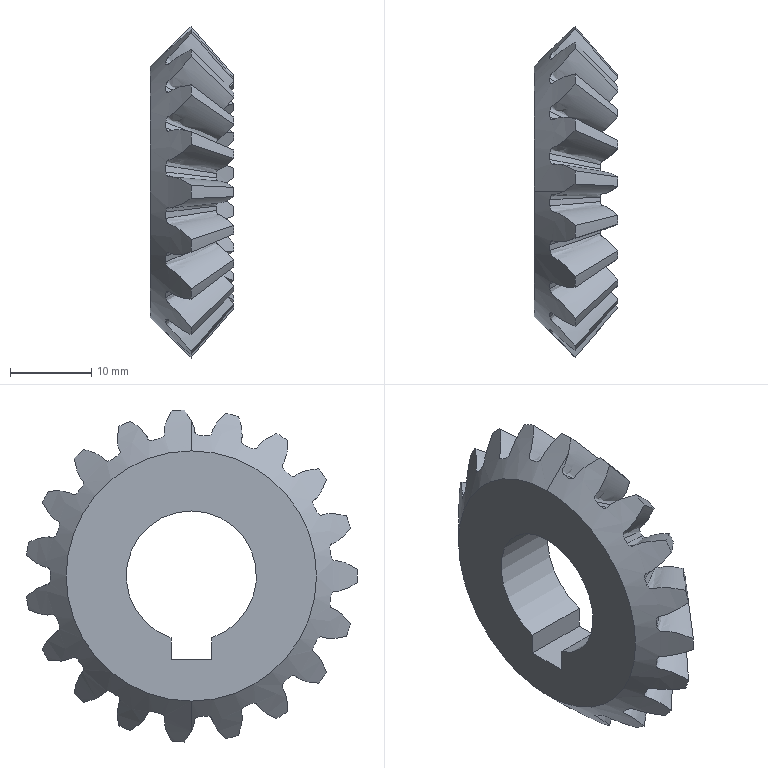Part | SolidWorks | features 3DProfileFeature 12, BlendCut 1, CirPattern 1, ICE 1, RefAxis 1, Revolution 1 | 1 solid | 86 faces | box 10.311 x 40.668 x 40.791 mm | volume 5692 mm3 | spline 38 | plane 24 | cone 23 | cylinder 1 | commonest cylinder face diameters 16 x1